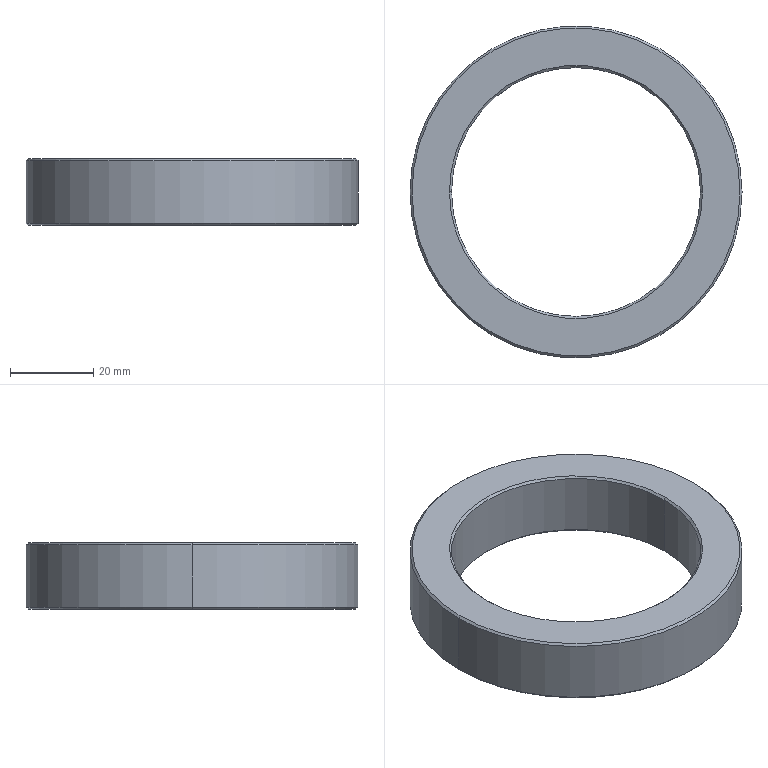Part | SolidWorks | features Chamfer 1, Extrusion 1 | 1 solid | 14 faces | box 80 x 80 x 16 mm | volume 35076 mm3 | cone 8 | cylinder 4 | plane 2 | commonest cylinder face diameters 60 x2 80 x2
STEP:
#1=CARTESIAN_POINT('',(39.5,0.,16.));
#2=VERTEX_POINT('',#1);
#3=CARTESIAN_POINT('',(-39.5,0.,16.));
#4=VERTEX_POINT('',#3);
#5=CARTESIAN_POINT('',(0.,0.,16.));
#6=DIRECTION('',(0.,0.,1.));
#7=DIRECTION('',(1.,0.,0.));
#8=AXIS2_PLACEMENT_3D('',#5,#6,#7);
#9=CIRCLE('',#8,39.5);
#10=EDGE_CURVE('',#2,#4,#9,.T.);
#11=ORIENTED_EDGE('',*,*,#10,.F.);
#12=CARTESIAN_POINT('',(40.,0.,15.5));
#13=VERTEX_POINT('',#12);
#14=CARTESIAN_POINT('',(39.5,0.,16.));
#15=DIRECTION('',(0.7071,0.,-0.7071));
#16=VECTOR('',#15,1000.);
#17=LINE('',#14,#16);
#18=EDGE_CURVE('',#2,#13,#17,.T.);
#19=ORIENTED_EDGE('',*,*,#18,.T.);
#20=CARTESIAN_POINT('',(-40.,0.,15.5));
#21=VERTEX_POINT('',#20);
#22=CARTESIAN_POINT('',(0.,0.,15.5));
#23=DIRECTION('',(0.,0.,-1.));
#24=DIRECTION('',(1.,0.,0.));
#25=AXIS2_PLACEMENT_3D('',#22,#23,#24);
#26=CIRCLE('',#25,40.);
#27=EDGE_CURVE('',#21,#13,#26,.T.);
#28=ORIENTED_EDGE('',*,*,#27,.F.);
#29=CARTESIAN_POINT('',(-39.5,0.,16.));
#30=DIRECTION('',(-0.7071,0.,-0.7071));
#31=VECTOR('',#30,1000.);
#32=LINE('',#29,#31);
#33=EDGE_CURVE('',#4,#21,#32,.T.);
#34=ORIENTED_EDGE('',*,*,#33,.F.);
#35=EDGE_LOOP('',(#11,#19,#28,#34));
#36=FACE_OUTER_BOUND('',#35,.T.);
#37=CARTESIAN_POINT('',(0.,0.,16.));
#38=DIRECTION('',(0.,0.,-1.));
#39=DIRECTION('',(-1.,0.,0.));
#40=AXIS2_PLACEMENT_3D('',#37,#38,#39);
#41=CONICAL_SURFACE('',#40,39.5,0.7854);
#42=ADVANCED_FACE('',(#36),#41,.T.);
#43=CARTESIAN_POINT('',(-30.,0.,15.5));
#44=VERTEX_POINT('',#43);
#45=CARTESIAN_POINT('',(30.,0.,15.5));
#46=VERTEX_POINT('',#45);
#47=CARTESIAN_POINT('',(0.,0.,15.5));
#48=DIRECTION('',(0.,0.,1.));
#49=DIRECTION('',(1.,0.,0.));
#50=AXIS2_PLACEMENT_3D('',#47,#48,#49);
#51=CIRCLE('',#50,30.);
#52=EDGE_CURVE('',#44,#46,#51,.T.);
#53=ORIENTED_EDGE('',*,*,#52,.F.);
#54=CARTESIAN_POINT('',(-30.5,0.,16.));
#55=VERTEX_POINT('',#54);
#56=CARTESIAN_POINT('',(-30.,0.,15.5));
#57=DIRECTION('',(-0.7071,0.,0.7071));
#58=VECTOR('',#57,1000.);
#59=LINE('',#56,#58);
#60=EDGE_CURVE('',#44,#55,#59,.T.);
#61=ORIENTED_EDGE('',*,*,#60,.T.);
#62=CARTESIAN_POINT('',(30.5,0.,16.));
#63=VERTEX_POINT('',#62);
#64=CARTESIAN_POINT('',(0.,0.,16.));
#65=DIRECTION('',(0.,0.,-1.));
#66=DIRECTION('',(1.,0.,0.));
#67=AXIS2_PLACEMENT_3D('',#64,#65,#66);
#68=CIRCLE('',#67,30.5);
#69=EDGE_CURVE('',#63,#55,#68,.T.);
#70=ORIENTED_EDGE('',*,*,#69,.F.);
#71=CARTESIAN_POINT('',(30.,0.,15.5));
#72=DIRECTION('',(0.7071,0.,0.7071));
#73=VECTOR('',#72,1000.);
#74=LINE('',#71,#73);
#75=EDGE_CURVE('',#46,#63,#74,.T.);
#76=ORIENTED_EDGE('',*,*,#75,.F.);
#77=EDGE_LOOP('',(#53,#61,#70,#76));
#78=FACE_OUTER_BOUND('',#77,.T.);
#79=CARTESIAN_POINT('',(0.,0.,15.5));
#80=DIRECTION('',(0.,0.,1.));
#81=DIRECTION('',(1.,0.,0.));
#82=AXIS2_PLACEMENT_3D('',#79,#80,#81);
#83=CONICAL_SURFACE('',#82,30.,0.7854);
#84=ADVANCED_FACE('',(#78),#83,.F.);
#85=CARTESIAN_POINT('',(-39.5,0.,0.));
#86=VERTEX_POINT('',#85);
#87=CARTESIAN_POINT('',(39.5,0.,0.));
#88=VERTEX_POINT('',#87);
#89=CARTESIAN_POINT('',(0.,0.,0.));
#90=DIRECTION('',(0.,0.,-1.));
#91=DIRECTION('',(1.,0.,0.));
#92=AXIS2_PLACEMENT_3D('',#89,#90,#91);
#93=CIRCLE('',#92,39.5);
#94=EDGE_CURVE('',#86,#88,#93,.T.);
#95=ORIENTED_EDGE('',*,*,#94,.F.);
#96=CARTESIAN_POINT('',(-40.,0.,0.5));
#97=VERTEX_POINT('',#96);
#98=CARTESIAN_POINT('',(-40.,0.,0.5));
#99=DIRECTION('',(-0.7071,0.,0.7071));
#100=VECTOR('',#99,1000.);
#101=LINE('',#98,#100);
#102=EDGE_CURVE('',#86,#97,#101,.T.);
#103=ORIENTED_EDGE('',*,*,#102,.T.);
#104=CARTESIAN_POINT('',(40.,0.,0.5));
#105=VERTEX_POINT('',#104);
#106=CARTESIAN_POINT('',(0.,0.,0.5));
#107=DIRECTION('',(0.,0.,1.));
#108=DIRECTION('',(1.,0.,0.));
#109=AXIS2_PLACEMENT_3D('',#106,#107,#108);
#110=CIRCLE('',#109,40.);
#111=EDGE_CURVE('',#105,#97,#110,.T.);
#112=ORIENTED_EDGE('',*,*,#111,.F.);
#113=CARTESIAN_POINT('',(40.,0.,0.5));
#114=DIRECTION('',(0.7071,0.,0.7071));
#115=VECTOR('',#114,1000.);
#116=LINE('',#113,#115);
#117=EDGE_CURVE('',#88,#105,#116,.T.);
#118=ORIENTED_EDGE('',*,*,#117,.F.);
#119=EDGE_LOOP('',(#95,#103,#112,#118));
#120=FACE_OUTER_BOUND('',#119,.T.);
#121=CARTESIAN_POINT('',(0.,0.,0.5));
#122=DIRECTION('',(0.,0.,1.));
#123=DIRECTION('',(1.,0.,0.));
#124=AXIS2_PLACEMENT_3D('',#121,#122,#123);
#125=CONICAL_SURFACE('',#124,40.,0.7854);
#126=ADVANCED_FACE('',(#120),#125,.T.);
#127=CARTESIAN_POINT('',(30.,0.,0.5));
#128=VERTEX_POINT('',#127);
#129=CARTESIAN_POINT('',(-30.,0.,0.5));
#130=VERTEX_POINT('',#129);
#131=CARTESIAN_POINT('',(0.,0.,0.5));
#132=DIRECTION('',(0.,0.,-1.));
#133=DIRECTION('',(1.,0.,0.));
#134=AXIS2_PLACEMENT_3D('',#131,#132,#133);
#135=CIRCLE('',#134,30.);
#136=EDGE_CURVE('',#128,#130,#135,.T.);
#137=ORIENTED_EDGE('',*,*,#136,.F.);
#138=CARTESIAN_POINT('',(30.5,0.,0.));
#139=VERTEX_POINT('',#138);
#140=CARTESIAN_POINT('',(30.5,0.,0.));
#141=DIRECTION('',(0.7071,0.,-0.7071));
#142=VECTOR('',#141,1000.);
#143=LINE('',#140,#142);
#144=EDGE_CURVE('',#128,#139,#143,.T.);
#145=ORIENTED_EDGE('',*,*,#144,.T.);
#146=CARTESIAN_POINT('',(-30.5,0.,0.));
#147=VERTEX_POINT('',#146);
#148=CARTESIAN_POINT('',(0.,0.,0.));
#149=DIRECTION('',(0.,0.,1.));
#150=DIRECTION('',(1.,0.,0.));
#151=AXIS2_PLACEMENT_3D('',#148,#149,#150);
#152=CIRCLE('',#151,30.5);
#153=EDGE_CURVE('',#147,#139,#152,.T.);
#154=ORIENTED_EDGE('',*,*,#153,.F.);
#155=CARTESIAN_POINT('',(-30.5,0.,0.));
#156=DIRECTION('',(-0.7071,0.,-0.7071));
#157=VECTOR('',#156,1000.);
#158=LINE('',#155,#157);
#159=EDGE_CURVE('',#130,#147,#158,.T.);
#160=ORIENTED_EDGE('',*,*,#159,.F.);
#161=EDGE_LOOP('',(#137,#145,#154,#160));
#162=FACE_OUTER_BOUND('',#161,.T.);
#163=CARTESIAN_POINT('',(0.,0.,0.));
#164=DIRECTION('',(0.,0.,-1.));
#165=DIRECTION('',(-1.,0.,0.));
#166=AXIS2_PLACEMENT_3D('',#163,#164,#165);
#167=CONICAL_SURFACE('',#166,30.5,0.7854);
#168=ADVANCED_FACE('',(#162),#167,.F.);
#169=ORIENTED_EDGE('',*,*,#52,.T.);
#170=CARTESIAN_POINT('',(30.,0.,16.));
#171=DIRECTION('',(0.,0.,-1.));
#172=VECTOR('',#171,1000.);
#173=LINE('',#170,#172);
#174=EDGE_CURVE('',#46,#128,#173,.T.);
#175=ORIENTED_EDGE('',*,*,#174,.T.);
#176=ORIENTED_EDGE('',*,*,#136,.T.);
#177=CARTESIAN_POINT('',(-30.,0.,16.));
#178=DIRECTION('',(0.,0.,-1.));
#179=VECTOR('',#178,1000.);
#180=LINE('',#177,#179);
#181=EDGE_CURVE('',#44,#130,#180,.T.);
#182=ORIENTED_EDGE('',*,*,#181,.F.);
#183=EDGE_LOOP('',(#169,#175,#176,#182));
#184=FACE_OUTER_BOUND('',#183,.T.);
#185=CARTESIAN_POINT('',(0.,0.,16.));
#186=DIRECTION('',(0.,0.,-1.));
#187=DIRECTION('',(-1.,0.,0.));
#188=AXIS2_PLACEMENT_3D('',#185,#186,#187);
#189=CYLINDRICAL_SURFACE('',#188,30.);
#190=ADVANCED_FACE('',(#184),#189,.F.);
#191=ORIENTED_EDGE('',*,*,#27,.T.);
#192=CARTESIAN_POINT('',(40.,0.,16.));
#193=DIRECTION('',(0.,0.,-1.));
#194=VECTOR('',#193,1000.);
#195=LINE('',#192,#194);
#196=EDGE_CURVE('',#13,#105,#195,.T.);
#197=ORIENTED_EDGE('',*,*,#196,.T.);
#198=ORIENTED_EDGE('',*,*,#111,.T.);
#199=CARTESIAN_POINT('',(-40.,0.,16.));
#200=DIRECTION('',(0.,0.,-1.));
#201=VECTOR('',#200,1000.);
#202=LINE('',#199,#201);
#203=EDGE_CURVE('',#21,#97,#202,.T.);
#204=ORIENTED_EDGE('',*,*,#203,.F.);
#205=EDGE_LOOP('',(#191,#197,#198,#204));
#206=FACE_OUTER_BOUND('',#205,.T.);
#207=CARTESIAN_POINT('',(0.,0.,16.));
#208=DIRECTION('',(0.,0.,-1.));
#209=DIRECTION('',(-1.,0.,0.));
#210=AXIS2_PLACEMENT_3D('',#207,#208,#209);
#211=CYLINDRICAL_SURFACE('',#210,40.);
#212=ADVANCED_FACE('',(#206),#211,.T.);
#213=ORIENTED_EDGE('',*,*,#69,.T.);
#214=CARTESIAN_POINT('',(0.,0.,16.));
#215=DIRECTION('',(0.,0.,-1.));
#216=DIRECTION('',(1.,0.,0.));
#217=AXIS2_PLACEMENT_3D('',#214,#215,#216);
#218=CIRCLE('',#217,30.5);
#219=EDGE_CURVE('',#55,#63,#218,.T.);
#220=ORIENTED_EDGE('',*,*,#219,.T.);
#221=EDGE_LOOP('',(#213,#220));
#222=FACE_BOUND('',#221,.T.);
#223=CARTESIAN_POINT('',(0.,0.,16.));
#224=DIRECTION('',(0.,0.,1.));
#225=DIRECTION('',(1.,0.,0.));
#226=AXIS2_PLACEMENT_3D('',#223,#224,#225);
#227=CIRCLE('',#226,39.5);
#228=EDGE_CURVE('',#4,#2,#227,.T.);
#229=ORIENTED_EDGE('',*,*,#228,.T.);
#230=ORIENTED_EDGE('',*,*,#10,.T.);
#231=EDGE_LOOP('',(#229,#230));
#232=FACE_OUTER_BOUND('',#231,.T.);
#233=CARTESIAN_POINT('',(0.,0.,16.));
#234=DIRECTION('',(0.,0.,1.));
#235=DIRECTION('',(1.,0.,0.));
#236=AXIS2_PLACEMENT_3D('',#233,#234,#235);
#237=PLANE('',#236);
#238=ADVANCED_FACE('',(#222,#232),#237,.T.);
#239=ORIENTED_EDGE('',*,*,#153,.T.);
#240=CARTESIAN_POINT('',(0.,0.,0.));
#241=DIRECTION('',(0.,0.,1.));
#242=DIRECTION('',(1.,0.,0.));
#243=AXIS2_PLACEMENT_3D('',#240,#241,#242);
#244=CIRCLE('',#243,30.5);
#245=EDGE_CURVE('',#139,#147,#244,.T.);
#246=ORIENTED_EDGE('',*,*,#245,.T.);
#247=EDGE_LOOP('',(#239,#246));
#248=FACE_BOUND('',#247,.T.);
#249=CARTESIAN_POINT('',(0.,0.,0.));
#250=DIRECTION('',(0.,0.,-1.));
#251=DIRECTION('',(1.,0.,0.));
#252=AXIS2_PLACEMENT_3D('',#249,#250,#251);
#253=CIRCLE('',#252,39.5);
#254=EDGE_CURVE('',#88,#86,#253,.T.);
#255=ORIENTED_EDGE('',*,*,#254,.T.);
#256=ORIENTED_EDGE('',*,*,#94,.T.);
#257=EDGE_LOOP('',(#255,#256));
#258=FACE_OUTER_BOUND('',#257,.T.);
#259=CARTESIAN_POINT('',(0.,0.,0.));
#260=DIRECTION('',(0.,0.,1.));
#261=DIRECTION('',(1.,0.,0.));
#262=AXIS2_PLACEMENT_3D('',#259,#260,#261);
#263=PLANE('',#262);
#264=ADVANCED_FACE('',(#248,#258),#263,.F.);
#265=ORIENTED_EDGE('',*,*,#196,.F.);
#266=CARTESIAN_POINT('',(0.,0.,15.5));
#267=DIRECTION('',(0.,0.,-1.));
#268=DIRECTION('',(1.,0.,0.));
#269=AXIS2_PLACEMENT_3D('',#266,#267,#268);
#270=CIRCLE('',#269,40.);
#271=EDGE_CURVE('',#13,#21,#270,.T.);
#272=ORIENTED_EDGE('',*,*,#271,.T.);
#273=ORIENTED_EDGE('',*,*,#203,.T.);
#274=CARTESIAN_POINT('',(0.,0.,0.5));
#275=DIRECTION('',(0.,0.,1.));
#276=DIRECTION('',(1.,0.,0.));
#277=AXIS2_PLACEMENT_3D('',#274,#275,#276);
#278=CIRCLE('',#277,40.);
#279=EDGE_CURVE('',#97,#105,#278,.T.);
#280=ORIENTED_EDGE('',*,*,#279,.T.);
#281=EDGE_LOOP('',(#265,#272,#273,#280));
#282=FACE_OUTER_BOUND('',#281,.T.);
#283=CARTESIAN_POINT('',(0.,0.,16.));
#284=DIRECTION('',(0.,0.,-1.));
#285=DIRECTION('',(-1.,0.,0.));
#286=AXIS2_PLACEMENT_3D('',#283,#284,#285);
#287=CYLINDRICAL_SURFACE('',#286,40.);
#288=ADVANCED_FACE('',(#282),#287,.T.);
#289=ORIENTED_EDGE('',*,*,#174,.F.);
#290=CARTESIAN_POINT('',(0.,0.,15.5));
#291=DIRECTION('',(0.,0.,1.));
#292=DIRECTION('',(1.,0.,0.));
#293=AXIS2_PLACEMENT_3D('',#290,#291,#292);
#294=CIRCLE('',#293,30.);
#295=EDGE_CURVE('',#46,#44,#294,.T.);
#296=ORIENTED_EDGE('',*,*,#295,.T.);
#297=ORIENTED_EDGE('',*,*,#181,.T.);
#298=CARTESIAN_POINT('',(0.,0.,0.5));
#299=DIRECTION('',(0.,0.,-1.));
#300=DIRECTION('',(1.,0.,0.));
#301=AXIS2_PLACEMENT_3D('',#298,#299,#300);
#302=CIRCLE('',#301,30.);
#303=EDGE_CURVE('',#130,#128,#302,.T.);
#304=ORIENTED_EDGE('',*,*,#303,.T.);
#305=EDGE_LOOP('',(#289,#296,#297,#304));
#306=FACE_OUTER_BOUND('',#305,.T.);
#307=CARTESIAN_POINT('',(0.,0.,16.));
#308=DIRECTION('',(0.,0.,-1.));
#309=DIRECTION('',(-1.,0.,0.));
#310=AXIS2_PLACEMENT_3D('',#307,#308,#309);
#311=CYLINDRICAL_SURFACE('',#310,30.);
#312=ADVANCED_FACE('',(#306),#311,.F.);
#313=ORIENTED_EDGE('',*,*,#144,.F.);
#314=ORIENTED_EDGE('',*,*,#303,.F.);
#315=ORIENTED_EDGE('',*,*,#159,.T.);
#316=ORIENTED_EDGE('',*,*,#245,.F.);
#317=EDGE_LOOP('',(#313,#314,#315,#316));
#318=FACE_OUTER_BOUND('',#317,.T.);
#319=CARTESIAN_POINT('',(0.,0.,0.));
#320=DIRECTION('',(0.,0.,-1.));
#321=DIRECTION('',(-1.,0.,0.));
#322=AXIS2_PLACEMENT_3D('',#319,#320,#321);
#323=CONICAL_SURFACE('',#322,30.5,0.7854);
#324=ADVANCED_FACE('',(#318),#323,.F.);
#325=ORIENTED_EDGE('',*,*,#102,.F.);
#326=ORIENTED_EDGE('',*,*,#254,.F.);
#327=ORIENTED_EDGE('',*,*,#117,.T.);
#328=ORIENTED_EDGE('',*,*,#279,.F.);
#329=EDGE_LOOP('',(#325,#326,#327,#328));
#330=FACE_OUTER_BOUND('',#329,.T.);
#331=CARTESIAN_POINT('',(0.,0.,0.5));
#332=DIRECTION('',(0.,0.,1.));
#333=DIRECTION('',(1.,0.,0.));
#334=AXIS2_PLACEMENT_3D('',#331,#332,#333);
#335=CONICAL_SURFACE('',#334,40.,0.7854);
#336=ADVANCED_FACE('',(#330),#335,.T.);
#337=ORIENTED_EDGE('',*,*,#60,.F.);
#338=ORIENTED_EDGE('',*,*,#295,.F.);
#339=ORIENTED_EDGE('',*,*,#75,.T.);
#340=ORIENTED_EDGE('',*,*,#219,.F.);
#341=EDGE_LOOP('',(#337,#338,#339,#340));
#342=FACE_OUTER_BOUND('',#341,.T.);
#343=CARTESIAN_POINT('',(0.,0.,15.5));
#344=DIRECTION('',(0.,0.,1.));
#345=DIRECTION('',(1.,0.,0.));
#346=AXIS2_PLACEMENT_3D('',#343,#344,#345);
#347=CONICAL_SURFACE('',#346,30.,0.7854);
#348=ADVANCED_FACE('',(#342),#347,.F.);
#349=ORIENTED_EDGE('',*,*,#18,.F.);
#350=ORIENTED_EDGE('',*,*,#228,.F.);
#351=ORIENTED_EDGE('',*,*,#33,.T.);
#352=ORIENTED_EDGE('',*,*,#271,.F.);
#353=EDGE_LOOP('',(#349,#350,#351,#352));
#354=FACE_OUTER_BOUND('',#353,.T.);
#355=CARTESIAN_POINT('',(0.,0.,16.));
#356=DIRECTION('',(0.,0.,-1.));
#357=DIRECTION('',(-1.,0.,0.));
#358=AXIS2_PLACEMENT_3D('',#355,#356,#357);
#359=CONICAL_SURFACE('',#358,39.5,0.7854);
#360=ADVANCED_FACE('',(#354),#359,.T.);
#361=CLOSED_SHELL('',(#42,#84,#126,#168,#190,#212,#238,#264,#288,#312,#324,#336,#348,#360));
#362=MANIFOLD_SOLID_BREP('',#361);
#363=CARTESIAN_POINT('',(0.,0.,0.));
#364=DIRECTION('',(0.,0.,1.));
#365=DIRECTION('',(1.,0.,0.));
#366=AXIS2_PLACEMENT_3D('',#363,#364,#365);
#367=(LENGTH_UNIT()NAMED_UNIT(*)SI_UNIT(.MILLI.,.METRE.));
#368=UNCERTAINTY_MEASURE_WITH_UNIT(LENGTH_MEASURE(0.00001),#367,'','');
#369=(NAMED_UNIT(*)PLANE_ANGLE_UNIT()SI_UNIT($,.RADIAN.));
#370=(NAMED_UNIT(*)SI_UNIT($,.STERADIAN.)SOLID_ANGLE_UNIT());
#371=(GEOMETRIC_REPRESENTATION_CONTEXT(3)GLOBAL_UNCERTAINTY_ASSIGNED_CONTEXT((#368))GLOBAL_UNIT_ASSIGNED_CONTEXT((#367,#369,#370))REPRESENTATION_CONTEXT('',''));
#372=ADVANCED_BREP_SHAPE_REPRESENTATION('',(#362,#366),#371);